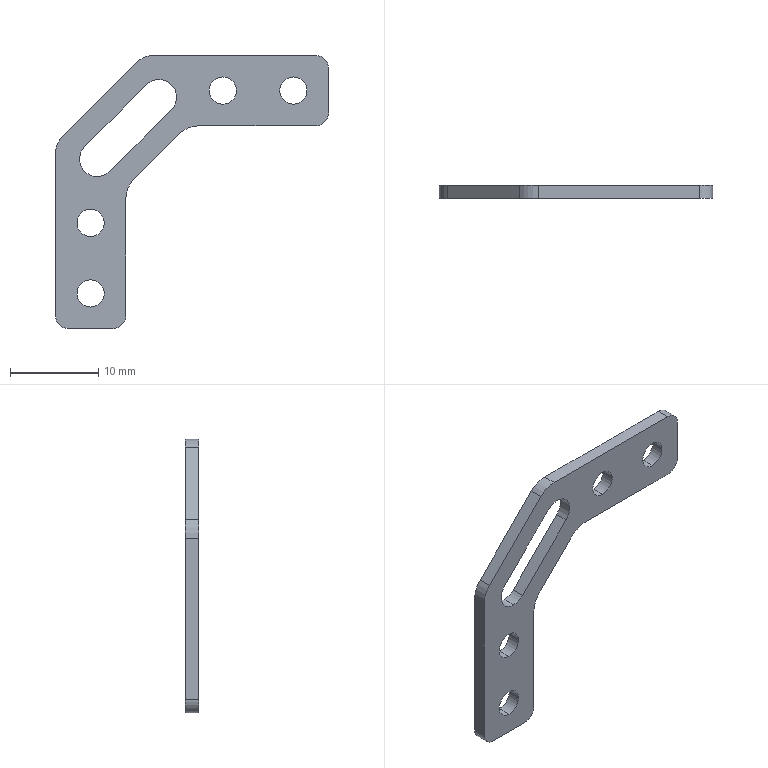Part | SolidWorks | features Fillet 2, Extrusion 1 | 1 solid | 31 faces | box 31 x 1.5 x 31 mm | volume 483.32 mm3 | cylinder 19 | plane 12 | commonest cylinder face diameters 3.1 x8 3 x4 6 x4 4 x3
STEP:
#1=CARTESIAN_POINT('',(2.164,1.5,-9.164));
#2=VERTEX_POINT('',#1);
#3=CARTESIAN_POINT('',(0.75,1.5,-9.75));
#4=VERTEX_POINT('',#3);
#5=CARTESIAN_POINT('',(0.75,1.5,-7.75));
#6=DIRECTION('',(0.,1.,0.));
#7=DIRECTION('',(0.,0.,1.));
#8=AXIS2_PLACEMENT_3D('',#5,#6,#7);
#9=CIRCLE('',#8,2.);
#10=EDGE_CURVE('',#2,#4,#9,.T.);
#11=ORIENTED_EDGE('',*,*,#10,.T.);
#12=CARTESIAN_POINT('',(0.75,0.,-9.75));
#13=VERTEX_POINT('',#12);
#14=CARTESIAN_POINT('',(0.75,1.5,-9.75));
#15=DIRECTION('',(0.,-1.,0.));
#16=VECTOR('',#15,1000.);
#17=LINE('',#14,#16);
#18=EDGE_CURVE('',#4,#13,#17,.T.);
#19=ORIENTED_EDGE('',*,*,#18,.T.);
#20=CARTESIAN_POINT('',(2.164,0.,-9.164));
#21=VERTEX_POINT('',#20);
#22=CARTESIAN_POINT('',(0.75,0.,-7.75));
#23=DIRECTION('',(0.,1.,0.));
#24=DIRECTION('',(0.,0.,1.));
#25=AXIS2_PLACEMENT_3D('',#22,#23,#24);
#26=CIRCLE('',#25,2.);
#27=EDGE_CURVE('',#21,#13,#26,.T.);
#28=ORIENTED_EDGE('',*,*,#27,.F.);
#29=CARTESIAN_POINT('',(2.164,1.5,-9.164));
#30=DIRECTION('',(0.,-1.,0.));
#31=VECTOR('',#30,1000.);
#32=LINE('',#29,#31);
#33=EDGE_CURVE('',#2,#21,#32,.T.);
#34=ORIENTED_EDGE('',*,*,#33,.F.);
#35=EDGE_LOOP('',(#11,#19,#28,#34));
#36=FACE_OUTER_BOUND('',#35,.T.);
#37=CARTESIAN_POINT('',(0.75,1.5,-7.75));
#38=DIRECTION('',(0.,-1.,0.));
#39=DIRECTION('',(0.,0.,-1.));
#40=AXIS2_PLACEMENT_3D('',#37,#38,#39);
#41=CYLINDRICAL_SURFACE('',#40,2.);
#42=ADVANCED_FACE('',(#36),#41,.F.);
#43=CARTESIAN_POINT('',(0.,1.5,-16.55));
#44=VERTEX_POINT('',#43);
#45=CARTESIAN_POINT('',(0.,1.5,-13.45));
#46=VERTEX_POINT('',#45);
#47=CARTESIAN_POINT('',(0.,1.5,-15.));
#48=DIRECTION('',(0.,1.,0.));
#49=DIRECTION('',(0.,0.,-1.));
#50=AXIS2_PLACEMENT_3D('',#47,#48,#49);
#51=CIRCLE('',#50,1.55);
#52=EDGE_CURVE('',#44,#46,#51,.T.);
#53=ORIENTED_EDGE('',*,*,#52,.T.);
#54=CARTESIAN_POINT('',(0.,0.,-13.45));
#55=VERTEX_POINT('',#54);
#56=CARTESIAN_POINT('',(0.,1.5,-13.45));
#57=DIRECTION('',(0.,-1.,0.));
#58=VECTOR('',#57,1000.);
#59=LINE('',#56,#58);
#60=EDGE_CURVE('',#46,#55,#59,.T.);
#61=ORIENTED_EDGE('',*,*,#60,.T.);
#62=CARTESIAN_POINT('',(0.,0.,-16.55));
#63=VERTEX_POINT('',#62);
#64=CARTESIAN_POINT('',(0.,0.,-15.));
#65=DIRECTION('',(0.,1.,0.));
#66=DIRECTION('',(0.,0.,-1.));
#67=AXIS2_PLACEMENT_3D('',#64,#65,#66);
#68=CIRCLE('',#67,1.55);
#69=EDGE_CURVE('',#63,#55,#68,.T.);
#70=ORIENTED_EDGE('',*,*,#69,.F.);
#71=CARTESIAN_POINT('',(0.,1.5,-16.55));
#72=DIRECTION('',(0.,-1.,0.));
#73=VECTOR('',#72,1000.);
#74=LINE('',#71,#73);
#75=EDGE_CURVE('',#44,#63,#74,.T.);
#76=ORIENTED_EDGE('',*,*,#75,.F.);
#77=EDGE_LOOP('',(#53,#61,#70,#76));
#78=FACE_OUTER_BOUND('',#77,.T.);
#79=CARTESIAN_POINT('',(0.,1.5,-15.));
#80=DIRECTION('',(0.,-1.,0.));
#81=DIRECTION('',(0.,0.,-1.));
#82=AXIS2_PLACEMENT_3D('',#79,#80,#81);
#83=CYLINDRICAL_SURFACE('',#82,1.55);
#84=ADVANCED_FACE('',(#78),#83,.F.);
#85=CARTESIAN_POINT('',(0.,1.5,-24.55));
#86=VERTEX_POINT('',#85);
#87=CARTESIAN_POINT('',(0.,1.5,-21.45));
#88=VERTEX_POINT('',#87);
#89=CARTESIAN_POINT('',(0.,1.5,-23.));
#90=DIRECTION('',(0.,1.,0.));
#91=DIRECTION('',(0.,0.,-1.));
#92=AXIS2_PLACEMENT_3D('',#89,#90,#91);
#93=CIRCLE('',#92,1.55);
#94=EDGE_CURVE('',#86,#88,#93,.T.);
#95=ORIENTED_EDGE('',*,*,#94,.T.);
#96=CARTESIAN_POINT('',(0.,0.,-21.45));
#97=VERTEX_POINT('',#96);
#98=CARTESIAN_POINT('',(0.,1.5,-21.45));
#99=DIRECTION('',(0.,-1.,0.));
#100=VECTOR('',#99,1000.);
#101=LINE('',#98,#100);
#102=EDGE_CURVE('',#88,#97,#101,.T.);
#103=ORIENTED_EDGE('',*,*,#102,.T.);
#104=CARTESIAN_POINT('',(0.,0.,-24.55));
#105=VERTEX_POINT('',#104);
#106=CARTESIAN_POINT('',(0.,0.,-23.));
#107=DIRECTION('',(0.,1.,0.));
#108=DIRECTION('',(0.,0.,-1.));
#109=AXIS2_PLACEMENT_3D('',#106,#107,#108);
#110=CIRCLE('',#109,1.55);
#111=EDGE_CURVE('',#105,#97,#110,.T.);
#112=ORIENTED_EDGE('',*,*,#111,.F.);
#113=CARTESIAN_POINT('',(0.,1.5,-24.55));
#114=DIRECTION('',(0.,-1.,0.));
#115=VECTOR('',#114,1000.);
#116=LINE('',#113,#115);
#117=EDGE_CURVE('',#86,#105,#116,.T.);
#118=ORIENTED_EDGE('',*,*,#117,.F.);
#119=EDGE_LOOP('',(#95,#103,#112,#118));
#120=FACE_OUTER_BOUND('',#119,.T.);
#121=CARTESIAN_POINT('',(0.,1.5,-23.));
#122=DIRECTION('',(0.,-1.,0.));
#123=DIRECTION('',(0.,0.,-1.));
#124=AXIS2_PLACEMENT_3D('',#121,#122,#123);
#125=CYLINDRICAL_SURFACE('',#124,1.55);
#126=ADVANCED_FACE('',(#120),#125,.F.);
#127=CARTESIAN_POINT('',(23.,1.5,-1.55));
#128=VERTEX_POINT('',#127);
#129=CARTESIAN_POINT('',(23.,1.5,1.55));
#130=VERTEX_POINT('',#129);
#131=CARTESIAN_POINT('',(23.,1.5,0.));
#132=DIRECTION('',(0.,1.,0.));
#133=DIRECTION('',(0.,0.,1.));
#134=AXIS2_PLACEMENT_3D('',#131,#132,#133);
#135=CIRCLE('',#134,1.55);
#136=EDGE_CURVE('',#128,#130,#135,.T.);
#137=ORIENTED_EDGE('',*,*,#136,.T.);
#138=CARTESIAN_POINT('',(23.,0.,1.55));
#139=VERTEX_POINT('',#138);
#140=CARTESIAN_POINT('',(23.,1.5,1.55));
#141=DIRECTION('',(0.,-1.,0.));
#142=VECTOR('',#141,1000.);
#143=LINE('',#140,#142);
#144=EDGE_CURVE('',#130,#139,#143,.T.);
#145=ORIENTED_EDGE('',*,*,#144,.T.);
#146=CARTESIAN_POINT('',(23.,0.,-1.55));
#147=VERTEX_POINT('',#146);
#148=CARTESIAN_POINT('',(23.,0.,0.));
#149=DIRECTION('',(0.,1.,0.));
#150=DIRECTION('',(0.,0.,1.));
#151=AXIS2_PLACEMENT_3D('',#148,#149,#150);
#152=CIRCLE('',#151,1.55);
#153=EDGE_CURVE('',#147,#139,#152,.T.);
#154=ORIENTED_EDGE('',*,*,#153,.F.);
#155=CARTESIAN_POINT('',(23.,1.5,-1.55));
#156=DIRECTION('',(0.,-1.,0.));
#157=VECTOR('',#156,1000.);
#158=LINE('',#155,#157);
#159=EDGE_CURVE('',#128,#147,#158,.T.);
#160=ORIENTED_EDGE('',*,*,#159,.F.);
#161=EDGE_LOOP('',(#137,#145,#154,#160));
#162=FACE_OUTER_BOUND('',#161,.T.);
#163=CARTESIAN_POINT('',(23.,1.5,0.));
#164=DIRECTION('',(0.,-1.,0.));
#165=DIRECTION('',(0.,0.,-1.));
#166=AXIS2_PLACEMENT_3D('',#163,#164,#165);
#167=CYLINDRICAL_SURFACE('',#166,1.55);
#168=ADVANCED_FACE('',(#162),#167,.F.);
#169=CARTESIAN_POINT('',(15.,1.5,-1.55));
#170=VERTEX_POINT('',#169);
#171=CARTESIAN_POINT('',(15.,1.5,1.55));
#172=VERTEX_POINT('',#171);
#173=CARTESIAN_POINT('',(15.,1.5,0.));
#174=DIRECTION('',(0.,1.,0.));
#175=DIRECTION('',(0.,0.,1.));
#176=AXIS2_PLACEMENT_3D('',#173,#174,#175);
#177=CIRCLE('',#176,1.55);
#178=EDGE_CURVE('',#170,#172,#177,.T.);
#179=ORIENTED_EDGE('',*,*,#178,.T.);
#180=CARTESIAN_POINT('',(15.,0.,1.55));
#181=VERTEX_POINT('',#180);
#182=CARTESIAN_POINT('',(15.,1.5,1.55));
#183=DIRECTION('',(0.,-1.,0.));
#184=VECTOR('',#183,1000.);
#185=LINE('',#182,#184);
#186=EDGE_CURVE('',#172,#181,#185,.T.);
#187=ORIENTED_EDGE('',*,*,#186,.T.);
#188=CARTESIAN_POINT('',(15.,0.,-1.55));
#189=VERTEX_POINT('',#188);
#190=CARTESIAN_POINT('',(15.,0.,0.));
#191=DIRECTION('',(0.,1.,0.));
#192=DIRECTION('',(0.,0.,1.));
#193=AXIS2_PLACEMENT_3D('',#190,#191,#192);
#194=CIRCLE('',#193,1.55);
#195=EDGE_CURVE('',#189,#181,#194,.T.);
#196=ORIENTED_EDGE('',*,*,#195,.F.);
#197=CARTESIAN_POINT('',(15.,1.5,-1.55));
#198=DIRECTION('',(0.,-1.,0.));
#199=VECTOR('',#198,1000.);
#200=LINE('',#197,#199);
#201=EDGE_CURVE('',#170,#189,#200,.T.);
#202=ORIENTED_EDGE('',*,*,#201,.F.);
#203=EDGE_LOOP('',(#179,#187,#196,#202));
#204=FACE_OUTER_BOUND('',#203,.T.);
#205=CARTESIAN_POINT('',(15.,1.5,0.));
#206=DIRECTION('',(0.,-1.,0.));
#207=DIRECTION('',(0.,0.,-1.));
#208=AXIS2_PLACEMENT_3D('',#205,#206,#207);
#209=CYLINDRICAL_SURFACE('',#208,1.55);
#210=ADVANCED_FACE('',(#204),#209,.F.);
#211=ORIENTED_EDGE('',*,*,#94,.F.);
#212=CARTESIAN_POINT('',(0.,1.5,-23.));
#213=DIRECTION('',(0.,1.,0.));
#214=DIRECTION('',(0.,0.,-1.));
#215=AXIS2_PLACEMENT_3D('',#212,#213,#214);
#216=CIRCLE('',#215,1.55);
#217=EDGE_CURVE('',#88,#86,#216,.T.);
#218=ORIENTED_EDGE('',*,*,#217,.F.);
#219=EDGE_LOOP('',(#211,#218));
#220=FACE_BOUND('',#219,.T.);
#221=ORIENTED_EDGE('',*,*,#178,.F.);
#222=CARTESIAN_POINT('',(15.,1.5,0.));
#223=DIRECTION('',(0.,1.,0.));
#224=DIRECTION('',(0.,0.,1.));
#225=AXIS2_PLACEMENT_3D('',#222,#223,#224);
#226=CIRCLE('',#225,1.55);
#227=EDGE_CURVE('',#172,#170,#226,.T.);
#228=ORIENTED_EDGE('',*,*,#227,.F.);
#229=EDGE_LOOP('',(#221,#228));
#230=FACE_BOUND('',#229,.T.);
#231=CARTESIAN_POINT('',(-3.121,1.5,-5.121));
#232=VERTEX_POINT('',#231);
#233=CARTESIAN_POINT('',(5.121,1.5,3.121));
#234=VERTEX_POINT('',#233);
#235=CARTESIAN_POINT('',(6.,1.5,4.));
#236=DIRECTION('',(0.7071,0.,0.7071));
#237=VECTOR('',#236,1000.);
#238=LINE('',#235,#237);
#239=EDGE_CURVE('',#232,#234,#238,.T.);
#240=ORIENTED_EDGE('',*,*,#239,.T.);
#241=CARTESIAN_POINT('',(7.243,1.5,4.));
#242=VERTEX_POINT('',#241);
#243=CARTESIAN_POINT('',(7.243,1.5,1.));
#244=DIRECTION('',(0.,1.,0.));
#245=DIRECTION('',(0.,0.,1.));
#246=AXIS2_PLACEMENT_3D('',#243,#244,#245);
#247=CIRCLE('',#246,3.);
#248=EDGE_CURVE('',#234,#242,#247,.T.);
#249=ORIENTED_EDGE('',*,*,#248,.T.);
#250=CARTESIAN_POINT('',(25.5,1.5,4.));
#251=VERTEX_POINT('',#250);
#252=CARTESIAN_POINT('',(27.,1.5,4.));
#253=DIRECTION('',(1.,0.,0.));
#254=VECTOR('',#253,1000.);
#255=LINE('',#252,#254);
#256=EDGE_CURVE('',#242,#251,#255,.T.);
#257=ORIENTED_EDGE('',*,*,#256,.T.);
#258=CARTESIAN_POINT('',(27.,1.5,2.5));
#259=VERTEX_POINT('',#258);
#260=CARTESIAN_POINT('',(25.5,1.5,2.5));
#261=DIRECTION('',(0.,1.,0.));
#262=DIRECTION('',(0.,0.,1.));
#263=AXIS2_PLACEMENT_3D('',#260,#261,#262);
#264=CIRCLE('',#263,1.5);
#265=EDGE_CURVE('',#251,#259,#264,.T.);
#266=ORIENTED_EDGE('',*,*,#265,.T.);
#267=CARTESIAN_POINT('',(27.,1.5,-2.5));
#268=VERTEX_POINT('',#267);
#269=CARTESIAN_POINT('',(27.,1.5,4.));
#270=DIRECTION('',(0.,0.,-1.));
#271=VECTOR('',#270,1000.);
#272=LINE('',#269,#271);
#273=EDGE_CURVE('',#259,#268,#272,.T.);
#274=ORIENTED_EDGE('',*,*,#273,.T.);
#275=CARTESIAN_POINT('',(25.5,1.5,-4.));
#276=VERTEX_POINT('',#275);
#277=CARTESIAN_POINT('',(25.5,1.5,-2.5));
#278=DIRECTION('',(0.,1.,0.));
#279=DIRECTION('',(0.,0.,1.));
#280=AXIS2_PLACEMENT_3D('',#277,#278,#279);
#281=CIRCLE('',#280,1.5);
#282=EDGE_CURVE('',#268,#276,#281,.T.);
#283=ORIENTED_EDGE('',*,*,#282,.T.);
#284=CARTESIAN_POINT('',(12.243,1.5,-4.));
#285=VERTEX_POINT('',#284);
#286=CARTESIAN_POINT('',(27.,1.5,-4.));
#287=DIRECTION('',(-1.,0.,0.));
#288=VECTOR('',#287,1000.);
#289=LINE('',#286,#288);
#290=EDGE_CURVE('',#276,#285,#289,.T.);
#291=ORIENTED_EDGE('',*,*,#290,.T.);
#292=CARTESIAN_POINT('',(10.121,1.5,-4.879));
#293=VERTEX_POINT('',#292);
#294=CARTESIAN_POINT('',(12.243,1.5,-7.));
#295=DIRECTION('',(0.,-1.,0.));
#296=DIRECTION('',(0.,0.,1.));
#297=AXIS2_PLACEMENT_3D('',#294,#295,#296);
#298=CIRCLE('',#297,3.);
#299=EDGE_CURVE('',#285,#293,#298,.T.);
#300=ORIENTED_EDGE('',*,*,#299,.T.);
#301=CARTESIAN_POINT('',(4.879,1.5,-10.121));
#302=VERTEX_POINT('',#301);
#303=CARTESIAN_POINT('',(11.,1.5,-4.));
#304=DIRECTION('',(-0.7071,0.,-0.7071));
#305=VECTOR('',#304,1000.);
#306=LINE('',#303,#305);
#307=EDGE_CURVE('',#293,#302,#306,.T.);
#308=ORIENTED_EDGE('',*,*,#307,.T.);
#309=CARTESIAN_POINT('',(4.,1.5,-12.243));
#310=VERTEX_POINT('',#309);
#311=CARTESIAN_POINT('',(7.,1.5,-12.243));
#312=DIRECTION('',(0.,-1.,0.));
#313=DIRECTION('',(0.,0.,1.));
#314=AXIS2_PLACEMENT_3D('',#311,#312,#313);
#315=CIRCLE('',#314,3.);
#316=EDGE_CURVE('',#302,#310,#315,.T.);
#317=ORIENTED_EDGE('',*,*,#316,.T.);
#318=CARTESIAN_POINT('',(4.,1.5,-25.5));
#319=VERTEX_POINT('',#318);
#320=CARTESIAN_POINT('',(4.,1.5,-27.));
#321=DIRECTION('',(0.,0.,-1.));
#322=VECTOR('',#321,1000.);
#323=LINE('',#320,#322);
#324=EDGE_CURVE('',#310,#319,#323,.T.);
#325=ORIENTED_EDGE('',*,*,#324,.T.);
#326=CARTESIAN_POINT('',(2.5,1.5,-27.));
#327=VERTEX_POINT('',#326);
#328=CARTESIAN_POINT('',(2.5,1.5,-25.5));
#329=DIRECTION('',(0.,1.,0.));
#330=DIRECTION('',(0.,0.,1.));
#331=AXIS2_PLACEMENT_3D('',#328,#329,#330);
#332=CIRCLE('',#331,1.5);
#333=EDGE_CURVE('',#319,#327,#332,.T.);
#334=ORIENTED_EDGE('',*,*,#333,.T.);
#335=CARTESIAN_POINT('',(-2.5,1.5,-27.));
#336=VERTEX_POINT('',#335);
#337=CARTESIAN_POINT('',(-4.,1.5,-27.));
#338=DIRECTION('',(-1.,0.,0.));
#339=VECTOR('',#338,1000.);
#340=LINE('',#337,#339);
#341=EDGE_CURVE('',#327,#336,#340,.T.);
#342=ORIENTED_EDGE('',*,*,#341,.T.);
#343=CARTESIAN_POINT('',(-4.,1.5,-25.5));
#344=VERTEX_POINT('',#343);
#345=CARTESIAN_POINT('',(-2.5,1.5,-25.5));
#346=DIRECTION('',(0.,1.,0.));
#347=DIRECTION('',(0.,0.,1.));
#348=AXIS2_PLACEMENT_3D('',#345,#346,#347);
#349=CIRCLE('',#348,1.5);
#350=EDGE_CURVE('',#336,#344,#349,.T.);
#351=ORIENTED_EDGE('',*,*,#350,.T.);
#352=CARTESIAN_POINT('',(-4.,1.5,-7.243));
#353=VERTEX_POINT('',#352);
#354=CARTESIAN_POINT('',(-4.,1.5,-27.));
#355=DIRECTION('',(0.,0.,1.));
#356=VECTOR('',#355,1000.);
#357=LINE('',#354,#356);
#358=EDGE_CURVE('',#344,#353,#357,.T.);
#359=ORIENTED_EDGE('',*,*,#358,.T.);
#360=CARTESIAN_POINT('',(-1.,1.5,-7.243));
#361=DIRECTION('',(0.,1.,0.));
#362=DIRECTION('',(0.,0.,1.));
#363=AXIS2_PLACEMENT_3D('',#360,#361,#362);
#364=CIRCLE('',#363,3.);
#365=EDGE_CURVE('',#353,#232,#364,.T.);
#366=ORIENTED_EDGE('',*,*,#365,.T.);
#367=EDGE_LOOP('',(#240,#249,#257,#266,#274,#283,#291,#300,#308,#317,#325,#334,#342,#351,#359,#366));
#368=FACE_OUTER_BOUND('',#367,.T.);
#369=ORIENTED_EDGE('',*,*,#136,.F.);
#370=CARTESIAN_POINT('',(23.,1.5,0.));
#371=DIRECTION('',(0.,1.,0.));
#372=DIRECTION('',(0.,0.,1.));
#373=AXIS2_PLACEMENT_3D('',#370,#371,#372);
#374=CIRCLE('',#373,1.55);
#375=EDGE_CURVE('',#130,#128,#374,.T.);
#376=ORIENTED_EDGE('',*,*,#375,.F.);
#377=EDGE_LOOP('',(#369,#376));
#378=FACE_BOUND('',#377,.T.);
#379=ORIENTED_EDGE('',*,*,#52,.F.);
#380=CARTESIAN_POINT('',(0.,1.5,-15.));
#381=DIRECTION('',(0.,1.,0.));
#382=DIRECTION('',(0.,0.,-1.));
#383=AXIS2_PLACEMENT_3D('',#380,#381,#382);
#384=CIRCLE('',#383,1.55);
#385=EDGE_CURVE('',#46,#44,#384,.T.);
#386=ORIENTED_EDGE('',*,*,#385,.F.);
#387=EDGE_LOOP('',(#379,#386));
#388=FACE_BOUND('',#387,.T.);
#389=CARTESIAN_POINT('',(-0.6642,1.5,-6.336));
#390=VERTEX_POINT('',#389);
#391=CARTESIAN_POINT('',(6.336,1.5,0.6642));
#392=VERTEX_POINT('',#391);
#393=CARTESIAN_POINT('',(-0.6642,1.5,-6.336));
#394=DIRECTION('',(0.7071,0.,0.7071));
#395=VECTOR('',#394,1000.);
#396=LINE('',#393,#395);
#397=EDGE_CURVE('',#390,#392,#396,.T.);
#398=ORIENTED_EDGE('',*,*,#397,.F.);
#399=CARTESIAN_POINT('',(0.75,1.5,-7.75));
#400=DIRECTION('',(0.,1.,0.));
#401=DIRECTION('',(0.,0.,1.));
#402=AXIS2_PLACEMENT_3D('',#399,#400,#401);
#403=CIRCLE('',#402,2.);
#404=EDGE_CURVE('',#4,#390,#403,.T.);
#405=ORIENTED_EDGE('',*,*,#404,.F.);
#406=ORIENTED_EDGE('',*,*,#10,.F.);
#407=CARTESIAN_POINT('',(9.164,1.5,-2.164));
#408=VERTEX_POINT('',#407);
#409=CARTESIAN_POINT('',(2.164,1.5,-9.164));
#410=DIRECTION('',(-0.7071,0.,-0.7071));
#411=VECTOR('',#410,1000.);
#412=LINE('',#409,#411);
#413=EDGE_CURVE('',#408,#2,#412,.T.);
#414=ORIENTED_EDGE('',*,*,#413,.F.);
#415=CARTESIAN_POINT('',(7.75,1.5,-0.75));
#416=DIRECTION('',(0.,1.,0.));
#417=DIRECTION('',(0.,0.,1.));
#418=AXIS2_PLACEMENT_3D('',#415,#416,#417);
#419=CIRCLE('',#418,2.);
#420=EDGE_CURVE('',#392,#408,#419,.T.);
#421=ORIENTED_EDGE('',*,*,#420,.F.);
#422=EDGE_LOOP('',(#398,#405,#406,#414,#421));
#423=FACE_BOUND('',#422,.T.);
#424=CARTESIAN_POINT('',(0.,1.5,0.));
#425=DIRECTION('',(0.,1.,0.));
#426=DIRECTION('',(0.,0.,1.));
#427=AXIS2_PLACEMENT_3D('',#424,#425,#426);
#428=PLANE('',#427);
#429=ADVANCED_FACE('',(#220,#230,#368,#378,#388,#423),#428,.T.);
#430=ORIENTED_EDGE('',*,*,#69,.T.);
#431=CARTESIAN_POINT('',(0.,0.,-15.));
#432=DIRECTION('',(0.,1.,0.));
#433=DIRECTION('',(0.,0.,-1.));
#434=AXIS2_PLACEMENT_3D('',#431,#432,#433);
#435=CIRCLE('',#434,1.55);
#436=EDGE_CURVE('',#55,#63,#435,.T.);
#437=ORIENTED_EDGE('',*,*,#436,.T.);
#438=EDGE_LOOP('',(#430,#437));
#439=FACE_BOUND('',#438,.T.);
#440=ORIENTED_EDGE('',*,*,#111,.T.);
#441=CARTESIAN_POINT('',(0.,0.,-23.));
#442=DIRECTION('',(0.,1.,0.));
#443=DIRECTION('',(0.,0.,-1.));
#444=AXIS2_PLACEMENT_3D('',#441,#442,#443);
#445=CIRCLE('',#444,1.55);
#446=EDGE_CURVE('',#97,#105,#445,.T.);
#447=ORIENTED_EDGE('',*,*,#446,.T.);
#448=EDGE_LOOP('',(#440,#447));
#449=FACE_BOUND('',#448,.T.);
#450=ORIENTED_EDGE('',*,*,#153,.T.);
#451=CARTESIAN_POINT('',(23.,0.,0.));
#452=DIRECTION('',(0.,1.,0.));
#453=DIRECTION('',(0.,0.,1.));
#454=AXIS2_PLACEMENT_3D('',#451,#452,#453);
#455=CIRCLE('',#454,1.55);
#456=EDGE_CURVE('',#139,#147,#455,.T.);
#457=ORIENTED_EDGE('',*,*,#456,.T.);
#458=EDGE_LOOP('',(#450,#457));
#459=FACE_BOUND('',#458,.T.);
#460=ORIENTED_EDGE('',*,*,#195,.T.);
#461=CARTESIAN_POINT('',(15.,0.,0.));
#462=DIRECTION('',(0.,1.,0.));
#463=DIRECTION('',(0.,0.,1.));
#464=AXIS2_PLACEMENT_3D('',#461,#462,#463);
#465=CIRCLE('',#464,1.55);
#466=EDGE_CURVE('',#181,#189,#465,.T.);
#467=ORIENTED_EDGE('',*,*,#466,.T.);
#468=EDGE_LOOP('',(#460,#467));
#469=FACE_BOUND('',#468,.T.);
#470=CARTESIAN_POINT('',(7.243,0.,4.));
#471=VERTEX_POINT('',#470);
#472=CARTESIAN_POINT('',(25.5,0.,4.));
#473=VERTEX_POINT('',#472);
#474=CARTESIAN_POINT('',(27.,0.,4.));
#475=DIRECTION('',(1.,0.,0.));
#476=VECTOR('',#475,1000.);
#477=LINE('',#474,#476);
#478=EDGE_CURVE('',#471,#473,#477,.T.);
#479=ORIENTED_EDGE('',*,*,#478,.F.);
#480=CARTESIAN_POINT('',(5.121,0.,3.121));
#481=VERTEX_POINT('',#480);
#482=CARTESIAN_POINT('',(7.243,0.,1.));
#483=DIRECTION('',(0.,-1.,0.));
#484=DIRECTION('',(0.,0.,1.));
#485=AXIS2_PLACEMENT_3D('',#482,#483,#484);
#486=CIRCLE('',#485,3.);
#487=EDGE_CURVE('',#471,#481,#486,.T.);
#488=ORIENTED_EDGE('',*,*,#487,.T.);
#489=CARTESIAN_POINT('',(-3.121,0.,-5.121));
#490=VERTEX_POINT('',#489);
#491=CARTESIAN_POINT('',(6.,0.,4.));
#492=DIRECTION('',(0.7071,0.,0.7071));
#493=VECTOR('',#492,1000.);
#494=LINE('',#491,#493);
#495=EDGE_CURVE('',#490,#481,#494,.T.);
#496=ORIENTED_EDGE('',*,*,#495,.F.);
#497=CARTESIAN_POINT('',(-4.,0.,-7.243));
#498=VERTEX_POINT('',#497);
#499=CARTESIAN_POINT('',(-1.,0.,-7.243));
#500=DIRECTION('',(0.,-1.,0.));
#501=DIRECTION('',(0.,0.,1.));
#502=AXIS2_PLACEMENT_3D('',#499,#500,#501);
#503=CIRCLE('',#502,3.);
#504=EDGE_CURVE('',#490,#498,#503,.T.);
#505=ORIENTED_EDGE('',*,*,#504,.T.);
#506=CARTESIAN_POINT('',(-4.,0.,-25.5));
#507=VERTEX_POINT('',#506);
#508=CARTESIAN_POINT('',(-4.,0.,-27.));
#509=DIRECTION('',(0.,0.,1.));
#510=VECTOR('',#509,1000.);
#511=LINE('',#508,#510);
#512=EDGE_CURVE('',#507,#498,#511,.T.);
#513=ORIENTED_EDGE('',*,*,#512,.F.);
#514=CARTESIAN_POINT('',(-2.5,0.,-27.));
#515=VERTEX_POINT('',#514);
#516=CARTESIAN_POINT('',(-2.5,0.,-25.5));
#517=DIRECTION('',(0.,-1.,0.));
#518=DIRECTION('',(0.,0.,1.));
#519=AXIS2_PLACEMENT_3D('',#516,#517,#518);
#520=CIRCLE('',#519,1.5);
#521=EDGE_CURVE('',#507,#515,#520,.T.);
#522=ORIENTED_EDGE('',*,*,#521,.T.);
#523=CARTESIAN_POINT('',(2.5,0.,-27.));
#524=VERTEX_POINT('',#523);
#525=CARTESIAN_POINT('',(-4.,0.,-27.));
#526=DIRECTION('',(-1.,0.,0.));
#527=VECTOR('',#526,1000.);
#528=LINE('',#525,#527);
#529=EDGE_CURVE('',#524,#515,#528,.T.);
#530=ORIENTED_EDGE('',*,*,#529,.F.);
#531=CARTESIAN_POINT('',(4.,0.,-25.5));
#532=VERTEX_POINT('',#531);
#533=CARTESIAN_POINT('',(2.5,0.,-25.5));
#534=DIRECTION('',(0.,-1.,0.));
#535=DIRECTION('',(0.,0.,1.));
#536=AXIS2_PLACEMENT_3D('',#533,#534,#535);
#537=CIRCLE('',#536,1.5);
#538=EDGE_CURVE('',#524,#532,#537,.T.);
#539=ORIENTED_EDGE('',*,*,#538,.T.);
#540=CARTESIAN_POINT('',(4.,0.,-12.243));
#541=VERTEX_POINT('',#540);
#542=CARTESIAN_POINT('',(4.,0.,-27.));
#543=DIRECTION('',(0.,0.,-1.));
#544=VECTOR('',#543,1000.);
#545=LINE('',#542,#544);
#546=EDGE_CURVE('',#541,#532,#545,.T.);
#547=ORIENTED_EDGE('',*,*,#546,.F.);
#548=CARTESIAN_POINT('',(4.879,0.,-10.121));
#549=VERTEX_POINT('',#548);
#550=CARTESIAN_POINT('',(7.,0.,-12.243));
#551=DIRECTION('',(0.,1.,0.));
#552=DIRECTION('',(0.,0.,1.));
#553=AXIS2_PLACEMENT_3D('',#550,#551,#552);
#554=CIRCLE('',#553,3.);
#555=EDGE_CURVE('',#541,#549,#554,.T.);
#556=ORIENTED_EDGE('',*,*,#555,.T.);
#557=CARTESIAN_POINT('',(10.121,0.,-4.879));
#558=VERTEX_POINT('',#557);
#559=CARTESIAN_POINT('',(11.,0.,-4.));
#560=DIRECTION('',(-0.7071,0.,-0.7071));
#561=VECTOR('',#560,1000.);
#562=LINE('',#559,#561);
#563=EDGE_CURVE('',#558,#549,#562,.T.);
#564=ORIENTED_EDGE('',*,*,#563,.F.);
#565=CARTESIAN_POINT('',(12.243,0.,-4.));
#566=VERTEX_POINT('',#565);
#567=CARTESIAN_POINT('',(12.243,0.,-7.));
#568=DIRECTION('',(0.,1.,0.));
#569=DIRECTION('',(0.,0.,1.));
#570=AXIS2_PLACEMENT_3D('',#567,#568,#569);
#571=CIRCLE('',#570,3.);
#572=EDGE_CURVE('',#558,#566,#571,.T.);
#573=ORIENTED_EDGE('',*,*,#572,.T.);
#574=CARTESIAN_POINT('',(25.5,0.,-4.));
#575=VERTEX_POINT('',#574);
#576=CARTESIAN_POINT('',(27.,0.,-4.));
#577=DIRECTION('',(-1.,0.,0.));
#578=VECTOR('',#577,1000.);
#579=LINE('',#576,#578);
#580=EDGE_CURVE('',#575,#566,#579,.T.);
#581=ORIENTED_EDGE('',*,*,#580,.F.);
#582=CARTESIAN_POINT('',(27.,0.,-2.5));
#583=VERTEX_POINT('',#582);
#584=CARTESIAN_POINT('',(25.5,0.,-2.5));
#585=DIRECTION('',(0.,-1.,0.));
#586=DIRECTION('',(0.,0.,1.));
#587=AXIS2_PLACEMENT_3D('',#584,#585,#586);
#588=CIRCLE('',#587,1.5);
#589=EDGE_CURVE('',#575,#583,#588,.T.);
#590=ORIENTED_EDGE('',*,*,#589,.T.);
#591=CARTESIAN_POINT('',(27.,0.,2.5));
#592=VERTEX_POINT('',#591);
#593=CARTESIAN_POINT('',(27.,0.,4.));
#594=DIRECTION('',(0.,0.,-1.));
#595=VECTOR('',#594,1000.);
#596=LINE('',#593,#595);
#597=EDGE_CURVE('',#592,#583,#596,.T.);
#598=ORIENTED_EDGE('',*,*,#597,.F.);
#599=CARTESIAN_POINT('',(25.5,0.,2.5));
#600=DIRECTION('',(0.,-1.,0.));
#601=DIRECTION('',(0.,0.,1.));
#602=AXIS2_PLACEMENT_3D('',#599,#600,#601);
#603=CIRCLE('',#602,1.5);
#604=EDGE_CURVE('',#592,#473,#603,.T.);
#605=ORIENTED_EDGE('',*,*,#604,.T.);
#606=EDGE_LOOP('',(#479,#488,#496,#505,#513,#522,#530,#539,#547,#556,#564,#573,#581,#590,#598,#605));
#607=FACE_OUTER_BOUND('',#606,.T.);
#608=ORIENTED_EDGE('',*,*,#27,.T.);
#609=CARTESIAN_POINT('',(-0.6642,0.,-6.336));
#610=VERTEX_POINT('',#609);
#611=CARTESIAN_POINT('',(0.75,0.,-7.75));
#612=DIRECTION('',(0.,1.,0.));
#613=DIRECTION('',(0.,0.,1.));
#614=AXIS2_PLACEMENT_3D('',#611,#612,#613);
#615=CIRCLE('',#614,2.);
#616=EDGE_CURVE('',#13,#610,#615,.T.);
#617=ORIENTED_EDGE('',*,*,#616,.T.);
#618=CARTESIAN_POINT('',(6.336,0.,0.6642));
#619=VERTEX_POINT('',#618);
#620=CARTESIAN_POINT('',(-0.6642,0.,-6.336));
#621=DIRECTION('',(0.7071,0.,0.7071));
#622=VECTOR('',#621,1000.);
#623=LINE('',#620,#622);
#624=EDGE_CURVE('',#610,#619,#623,.T.);
#625=ORIENTED_EDGE('',*,*,#624,.T.);
#626=CARTESIAN_POINT('',(9.164,0.,-2.164));
#627=VERTEX_POINT('',#626);
#628=CARTESIAN_POINT('',(7.75,0.,-0.75));
#629=DIRECTION('',(0.,1.,0.));
#630=DIRECTION('',(0.,0.,1.));
#631=AXIS2_PLACEMENT_3D('',#628,#629,#630);
#632=CIRCLE('',#631,2.);
#633=EDGE_CURVE('',#619,#627,#632,.T.);
#634=ORIENTED_EDGE('',*,*,#633,.T.);
#635=CARTESIAN_POINT('',(2.164,0.,-9.164));
#636=DIRECTION('',(-0.7071,0.,-0.7071));
#637=VECTOR('',#636,1000.);
#638=LINE('',#635,#637);
#639=EDGE_CURVE('',#627,#21,#638,.T.);
#640=ORIENTED_EDGE('',*,*,#639,.T.);
#641=EDGE_LOOP('',(#608,#617,#625,#634,#640));
#642=FACE_BOUND('',#641,.T.);
#643=CARTESIAN_POINT('',(0.,0.,0.));
#644=DIRECTION('',(0.,1.,0.));
#645=DIRECTION('',(0.,0.,1.));
#646=AXIS2_PLACEMENT_3D('',#643,#644,#645);
#647=PLANE('',#646);
#648=ADVANCED_FACE('',(#439,#449,#459,#469,#607,#642),#647,.F.);
#649=ORIENTED_EDGE('',*,*,#256,.F.);
#650=CARTESIAN_POINT('',(7.243,1.5,4.));
#651=DIRECTION('',(0.,-1.,0.));
#652=VECTOR('',#651,1000.);
#653=LINE('',#650,#652);
#654=EDGE_CURVE('',#242,#471,#653,.T.);
#655=ORIENTED_EDGE('',*,*,#654,.T.);
#656=ORIENTED_EDGE('',*,*,#478,.T.);
#657=CARTESIAN_POINT('',(25.5,1.5,4.));
#658=DIRECTION('',(0.,1.,0.));
#659=VECTOR('',#658,1000.);
#660=LINE('',#657,#659);
#661=EDGE_CURVE('',#473,#251,#660,.T.);
#662=ORIENTED_EDGE('',*,*,#661,.T.);
#663=EDGE_LOOP('',(#649,#655,#656,#662));
#664=FACE_OUTER_BOUND('',#663,.T.);
#665=CARTESIAN_POINT('',(27.,1.5,4.));
#666=DIRECTION('',(0.,0.,-1.));
#667=DIRECTION('',(-1.,0.,0.));
#668=AXIS2_PLACEMENT_3D('',#665,#666,#667);
#669=PLANE('',#668);
#670=ADVANCED_FACE('',(#664),#669,.F.);
#671=ORIENTED_EDGE('',*,*,#273,.F.);
#672=CARTESIAN_POINT('',(27.,1.5,2.5));
#673=DIRECTION('',(0.,-1.,0.));
#674=VECTOR('',#673,1000.);
#675=LINE('',#672,#674);
#676=EDGE_CURVE('',#259,#592,#675,.T.);
#677=ORIENTED_EDGE('',*,*,#676,.T.);
#678=ORIENTED_EDGE('',*,*,#597,.T.);
#679=CARTESIAN_POINT('',(27.,1.5,-2.5));
#680=DIRECTION('',(0.,1.,0.));
#681=VECTOR('',#680,1000.);
#682=LINE('',#679,#681);
#683=EDGE_CURVE('',#583,#268,#682,.T.);
#684=ORIENTED_EDGE('',*,*,#683,.T.);
#685=EDGE_LOOP('',(#671,#677,#678,#684));
#686=FACE_OUTER_BOUND('',#685,.T.);
#687=CARTESIAN_POINT('',(27.,1.5,4.));
#688=DIRECTION('',(-1.,0.,0.));
#689=DIRECTION('',(0.,0.,1.));
#690=AXIS2_PLACEMENT_3D('',#687,#688,#689);
#691=PLANE('',#690);
#692=ADVANCED_FACE('',(#686),#691,.F.);
#693=ORIENTED_EDGE('',*,*,#580,.T.);
#694=CARTESIAN_POINT('',(12.243,1.5,-4.));
#695=DIRECTION('',(0.,1.,0.));
#696=VECTOR('',#695,1000.);
#697=LINE('',#694,#696);
#698=EDGE_CURVE('',#566,#285,#697,.T.);
#699=ORIENTED_EDGE('',*,*,#698,.T.);
#700=ORIENTED_EDGE('',*,*,#290,.F.);
#701=CARTESIAN_POINT('',(25.5,1.5,-4.));
#702=DIRECTION('',(0.,-1.,0.));
#703=VECTOR('',#702,1000.);
#704=LINE('',#701,#703);
#705=EDGE_CURVE('',#276,#575,#704,.T.);
#706=ORIENTED_EDGE('',*,*,#705,.T.);
#707=EDGE_LOOP('',(#693,#699,#700,#706));
#708=FACE_OUTER_BOUND('',#707,.T.);
#709=CARTESIAN_POINT('',(27.,1.5,-4.));
#710=DIRECTION('',(0.,0.,1.));
#711=DIRECTION('',(1.,0.,0.));
#712=AXIS2_PLACEMENT_3D('',#709,#710,#711);
#713=PLANE('',#712);
#714=ADVANCED_FACE('',(#708),#713,.F.);
#715=ORIENTED_EDGE('',*,*,#563,.T.);
#716=CARTESIAN_POINT('',(4.879,1.5,-10.121));
#717=DIRECTION('',(0.,1.,0.));
#718=VECTOR('',#717,1000.);
#719=LINE('',#716,#718);
#720=EDGE_CURVE('',#549,#302,#719,.T.);
#721=ORIENTED_EDGE('',*,*,#720,.T.);
#722=ORIENTED_EDGE('',*,*,#307,.F.);
#723=CARTESIAN_POINT('',(10.121,0.,-4.879));
#724=DIRECTION('',(0.,-1.,0.));
#725=VECTOR('',#724,1000.);
#726=LINE('',#723,#725);
#727=EDGE_CURVE('',#293,#558,#726,.T.);
#728=ORIENTED_EDGE('',*,*,#727,.T.);
#729=EDGE_LOOP('',(#715,#721,#722,#728));
#730=FACE_OUTER_BOUND('',#729,.T.);
#731=CARTESIAN_POINT('',(11.,1.5,-4.));
#732=DIRECTION('',(-0.7071,0.,0.7071));
#733=DIRECTION('',(0.7071,0.,0.7071));
#734=AXIS2_PLACEMENT_3D('',#731,#732,#733);
#735=PLANE('',#734);
#736=ADVANCED_FACE('',(#730),#735,.F.);
#737=ORIENTED_EDGE('',*,*,#324,.F.);
#738=CARTESIAN_POINT('',(4.,0.,-12.243));
#739=DIRECTION('',(0.,-1.,0.));
#740=VECTOR('',#739,1000.);
#741=LINE('',#738,#740);
#742=EDGE_CURVE('',#310,#541,#741,.T.);
#743=ORIENTED_EDGE('',*,*,#742,.T.);
#744=ORIENTED_EDGE('',*,*,#546,.T.);
#745=CARTESIAN_POINT('',(4.,1.5,-25.5));
#746=DIRECTION('',(0.,1.,0.));
#747=VECTOR('',#746,1000.);
#748=LINE('',#745,#747);
#749=EDGE_CURVE('',#532,#319,#748,.T.);
#750=ORIENTED_EDGE('',*,*,#749,.T.);
#751=EDGE_LOOP('',(#737,#743,#744,#750));
#752=FACE_OUTER_BOUND('',#751,.T.);
#753=CARTESIAN_POINT('',(4.,1.5,-27.));
#754=DIRECTION('',(-1.,0.,0.));
#755=DIRECTION('',(0.,0.,1.));
#756=AXIS2_PLACEMENT_3D('',#753,#754,#755);
#757=PLANE('',#756);
#758=ADVANCED_FACE('',(#752),#757,.F.);
#759=ORIENTED_EDGE('',*,*,#341,.F.);
#760=CARTESIAN_POINT('',(2.5,1.5,-27.));
#761=DIRECTION('',(0.,-1.,0.));
#762=VECTOR('',#761,1000.);
#763=LINE('',#760,#762);
#764=EDGE_CURVE('',#327,#524,#763,.T.);
#765=ORIENTED_EDGE('',*,*,#764,.T.);
#766=ORIENTED_EDGE('',*,*,#529,.T.);
#767=CARTESIAN_POINT('',(-2.5,1.5,-27.));
#768=DIRECTION('',(0.,1.,0.));
#769=VECTOR('',#768,1000.);
#770=LINE('',#767,#769);
#771=EDGE_CURVE('',#515,#336,#770,.T.);
#772=ORIENTED_EDGE('',*,*,#771,.T.);
#773=EDGE_LOOP('',(#759,#765,#766,#772));
#774=FACE_OUTER_BOUND('',#773,.T.);
#775=CARTESIAN_POINT('',(-4.,1.5,-27.));
#776=DIRECTION('',(0.,0.,1.));
#777=DIRECTION('',(1.,0.,0.));
#778=AXIS2_PLACEMENT_3D('',#775,#776,#777);
#779=PLANE('',#778);
#780=ADVANCED_FACE('',(#774),#779,.F.);
#781=ORIENTED_EDGE('',*,*,#512,.T.);
#782=CARTESIAN_POINT('',(-4.,1.5,-7.243));
#783=DIRECTION('',(0.,1.,0.));
#784=VECTOR('',#783,1000.);
#785=LINE('',#782,#784);
#786=EDGE_CURVE('',#498,#353,#785,.T.);
#787=ORIENTED_EDGE('',*,*,#786,.T.);
#788=ORIENTED_EDGE('',*,*,#358,.F.);
#789=CARTESIAN_POINT('',(-4.,1.5,-25.5));
#790=DIRECTION('',(0.,-1.,0.));
#791=VECTOR('',#790,1000.);
#792=LINE('',#789,#791);
#793=EDGE_CURVE('',#344,#507,#792,.T.);
#794=ORIENTED_EDGE('',*,*,#793,.T.);
#795=EDGE_LOOP('',(#781,#787,#788,#794));
#796=FACE_OUTER_BOUND('',#795,.T.);
#797=CARTESIAN_POINT('',(-4.,1.5,-27.));
#798=DIRECTION('',(1.,0.,0.));
#799=DIRECTION('',(0.,0.,-1.));
#800=AXIS2_PLACEMENT_3D('',#797,#798,#799);
#801=PLANE('',#800);
#802=ADVANCED_FACE('',(#796),#801,.F.);
#803=ORIENTED_EDGE('',*,*,#495,.T.);
#804=CARTESIAN_POINT('',(5.121,1.5,3.121));
#805=DIRECTION('',(0.,1.,0.));
#806=VECTOR('',#805,1000.);
#807=LINE('',#804,#806);
#808=EDGE_CURVE('',#481,#234,#807,.T.);
#809=ORIENTED_EDGE('',*,*,#808,.T.);
#810=ORIENTED_EDGE('',*,*,#239,.F.);
#811=CARTESIAN_POINT('',(-3.121,1.5,-5.121));
#812=DIRECTION('',(0.,-1.,0.));
#813=VECTOR('',#812,1000.);
#814=LINE('',#811,#813);
#815=EDGE_CURVE('',#232,#490,#814,.T.);
#816=ORIENTED_EDGE('',*,*,#815,.T.);
#817=EDGE_LOOP('',(#803,#809,#810,#816));
#818=FACE_OUTER_BOUND('',#817,.T.);
#819=CARTESIAN_POINT('',(6.,1.5,4.));
#820=DIRECTION('',(0.7071,0.,-0.7071));
#821=DIRECTION('',(-0.7071,0.,-0.7071));
#822=AXIS2_PLACEMENT_3D('',#819,#820,#821);
#823=PLANE('',#822);
#824=ADVANCED_FACE('',(#818),#823,.F.);
#825=ORIENTED_EDGE('',*,*,#186,.F.);
#826=ORIENTED_EDGE('',*,*,#227,.T.);
#827=ORIENTED_EDGE('',*,*,#201,.T.);
#828=ORIENTED_EDGE('',*,*,#466,.F.);
#829=EDGE_LOOP('',(#825,#826,#827,#828));
#830=FACE_OUTER_BOUND('',#829,.T.);
#831=CARTESIAN_POINT('',(15.,1.5,0.));
#832=DIRECTION('',(0.,-1.,0.));
#833=DIRECTION('',(0.,0.,-1.));
#834=AXIS2_PLACEMENT_3D('',#831,#832,#833);
#835=CYLINDRICAL_SURFACE('',#834,1.55);
#836=ADVANCED_FACE('',(#830),#835,.F.);
#837=ORIENTED_EDGE('',*,*,#144,.F.);
#838=ORIENTED_EDGE('',*,*,#375,.T.);
#839=ORIENTED_EDGE('',*,*,#159,.T.);
#840=ORIENTED_EDGE('',*,*,#456,.F.);
#841=EDGE_LOOP('',(#837,#838,#839,#840));
#842=FACE_OUTER_BOUND('',#841,.T.);
#843=CARTESIAN_POINT('',(23.,1.5,0.));
#844=DIRECTION('',(0.,-1.,0.));
#845=DIRECTION('',(0.,0.,-1.));
#846=AXIS2_PLACEMENT_3D('',#843,#844,#845);
#847=CYLINDRICAL_SURFACE('',#846,1.55);
#848=ADVANCED_FACE('',(#842),#847,.F.);
#849=ORIENTED_EDGE('',*,*,#102,.F.);
#850=ORIENTED_EDGE('',*,*,#217,.T.);
#851=ORIENTED_EDGE('',*,*,#117,.T.);
#852=ORIENTED_EDGE('',*,*,#446,.F.);
#853=EDGE_LOOP('',(#849,#850,#851,#852));
#854=FACE_OUTER_BOUND('',#853,.T.);
#855=CARTESIAN_POINT('',(0.,1.5,-23.));
#856=DIRECTION('',(0.,-1.,0.));
#857=DIRECTION('',(0.,0.,-1.));
#858=AXIS2_PLACEMENT_3D('',#855,#856,#857);
#859=CYLINDRICAL_SURFACE('',#858,1.55);
#860=ADVANCED_FACE('',(#854),#859,.F.);
#861=ORIENTED_EDGE('',*,*,#60,.F.);
#862=ORIENTED_EDGE('',*,*,#385,.T.);
#863=ORIENTED_EDGE('',*,*,#75,.T.);
#864=ORIENTED_EDGE('',*,*,#436,.F.);
#865=EDGE_LOOP('',(#861,#862,#863,#864));
#866=FACE_OUTER_BOUND('',#865,.T.);
#867=CARTESIAN_POINT('',(0.,1.5,-15.));
#868=DIRECTION('',(0.,-1.,0.));
#869=DIRECTION('',(0.,0.,-1.));
#870=AXIS2_PLACEMENT_3D('',#867,#868,#869);
#871=CYLINDRICAL_SURFACE('',#870,1.55);
#872=ADVANCED_FACE('',(#866),#871,.F.);
#873=ORIENTED_EDGE('',*,*,#18,.F.);
#874=ORIENTED_EDGE('',*,*,#404,.T.);
#875=CARTESIAN_POINT('',(-0.6642,1.5,-6.336));
#876=DIRECTION('',(0.,-1.,0.));
#877=VECTOR('',#876,1000.);
#878=LINE('',#875,#877);
#879=EDGE_CURVE('',#390,#610,#878,.T.);
#880=ORIENTED_EDGE('',*,*,#879,.T.);
#881=ORIENTED_EDGE('',*,*,#616,.F.);
#882=EDGE_LOOP('',(#873,#874,#880,#881));
#883=FACE_OUTER_BOUND('',#882,.T.);
#884=CARTESIAN_POINT('',(0.75,1.5,-7.75));
#885=DIRECTION('',(0.,-1.,0.));
#886=DIRECTION('',(0.,0.,-1.));
#887=AXIS2_PLACEMENT_3D('',#884,#885,#886);
#888=CYLINDRICAL_SURFACE('',#887,2.);
#889=ADVANCED_FACE('',(#883),#888,.F.);
#890=ORIENTED_EDGE('',*,*,#624,.F.);
#891=ORIENTED_EDGE('',*,*,#879,.F.);
#892=ORIENTED_EDGE('',*,*,#397,.T.);
#893=CARTESIAN_POINT('',(6.336,1.5,0.6642));
#894=DIRECTION('',(0.,-1.,0.));
#895=VECTOR('',#894,1000.);
#896=LINE('',#893,#895);
#897=EDGE_CURVE('',#392,#619,#896,.T.);
#898=ORIENTED_EDGE('',*,*,#897,.T.);
#899=EDGE_LOOP('',(#890,#891,#892,#898));
#900=FACE_OUTER_BOUND('',#899,.T.);
#901=CARTESIAN_POINT('',(-0.6642,1.5,-6.336));
#902=DIRECTION('',(0.7071,0.,-0.7071));
#903=DIRECTION('',(-0.7071,0.,-0.7071));
#904=AXIS2_PLACEMENT_3D('',#901,#902,#903);
#905=PLANE('',#904);
#906=ADVANCED_FACE('',(#900),#905,.T.);
#907=ORIENTED_EDGE('',*,*,#633,.F.);
#908=ORIENTED_EDGE('',*,*,#897,.F.);
#909=ORIENTED_EDGE('',*,*,#420,.T.);
#910=CARTESIAN_POINT('',(9.164,1.5,-2.164));
#911=DIRECTION('',(0.,-1.,0.));
#912=VECTOR('',#911,1000.);
#913=LINE('',#910,#912);
#914=EDGE_CURVE('',#408,#627,#913,.T.);
#915=ORIENTED_EDGE('',*,*,#914,.T.);
#916=EDGE_LOOP('',(#907,#908,#909,#915));
#917=FACE_OUTER_BOUND('',#916,.T.);
#918=CARTESIAN_POINT('',(7.75,1.5,-0.75));
#919=DIRECTION('',(0.,-1.,0.));
#920=DIRECTION('',(0.,0.,-1.));
#921=AXIS2_PLACEMENT_3D('',#918,#919,#920);
#922=CYLINDRICAL_SURFACE('',#921,2.);
#923=ADVANCED_FACE('',(#917),#922,.F.);
#924=ORIENTED_EDGE('',*,*,#639,.F.);
#925=ORIENTED_EDGE('',*,*,#914,.F.);
#926=ORIENTED_EDGE('',*,*,#413,.T.);
#927=ORIENTED_EDGE('',*,*,#33,.T.);
#928=EDGE_LOOP('',(#924,#925,#926,#927));
#929=FACE_OUTER_BOUND('',#928,.T.);
#930=CARTESIAN_POINT('',(2.164,1.5,-9.164));
#931=DIRECTION('',(-0.7071,0.,0.7071));
#932=DIRECTION('',(0.7071,0.,0.7071));
#933=AXIS2_PLACEMENT_3D('',#930,#931,#932);
#934=PLANE('',#933);
#935=ADVANCED_FACE('',(#929),#934,.T.);
#936=ORIENTED_EDGE('',*,*,#265,.F.);
#937=ORIENTED_EDGE('',*,*,#661,.F.);
#938=ORIENTED_EDGE('',*,*,#604,.F.);
#939=ORIENTED_EDGE('',*,*,#676,.F.);
#940=EDGE_LOOP('',(#936,#937,#938,#939));
#941=FACE_OUTER_BOUND('',#940,.T.);
#942=CARTESIAN_POINT('',(25.5,1.5,2.5));
#943=DIRECTION('',(0.,-1.,0.));
#944=DIRECTION('',(0.,0.,-1.));
#945=AXIS2_PLACEMENT_3D('',#942,#943,#944);
#946=CYLINDRICAL_SURFACE('',#945,1.5);
#947=ADVANCED_FACE('',(#941),#946,.T.);
#948=ORIENTED_EDGE('',*,*,#282,.F.);
#949=ORIENTED_EDGE('',*,*,#683,.F.);
#950=ORIENTED_EDGE('',*,*,#589,.F.);
#951=ORIENTED_EDGE('',*,*,#705,.F.);
#952=EDGE_LOOP('',(#948,#949,#950,#951));
#953=FACE_OUTER_BOUND('',#952,.T.);
#954=CARTESIAN_POINT('',(25.5,1.5,-2.5));
#955=DIRECTION('',(0.,-1.,0.));
#956=DIRECTION('',(0.,0.,-1.));
#957=AXIS2_PLACEMENT_3D('',#954,#955,#956);
#958=CYLINDRICAL_SURFACE('',#957,1.5);
#959=ADVANCED_FACE('',(#953),#958,.T.);
#960=ORIENTED_EDGE('',*,*,#333,.F.);
#961=ORIENTED_EDGE('',*,*,#749,.F.);
#962=ORIENTED_EDGE('',*,*,#538,.F.);
#963=ORIENTED_EDGE('',*,*,#764,.F.);
#964=EDGE_LOOP('',(#960,#961,#962,#963));
#965=FACE_OUTER_BOUND('',#964,.T.);
#966=CARTESIAN_POINT('',(2.5,1.5,-25.5));
#967=DIRECTION('',(0.,-1.,0.));
#968=DIRECTION('',(0.,0.,-1.));
#969=AXIS2_PLACEMENT_3D('',#966,#967,#968);
#970=CYLINDRICAL_SURFACE('',#969,1.5);
#971=ADVANCED_FACE('',(#965),#970,.T.);
#972=ORIENTED_EDGE('',*,*,#350,.F.);
#973=ORIENTED_EDGE('',*,*,#771,.F.);
#974=ORIENTED_EDGE('',*,*,#521,.F.);
#975=ORIENTED_EDGE('',*,*,#793,.F.);
#976=EDGE_LOOP('',(#972,#973,#974,#975));
#977=FACE_OUTER_BOUND('',#976,.T.);
#978=CARTESIAN_POINT('',(-2.5,1.5,-25.5));
#979=DIRECTION('',(0.,-1.,0.));
#980=DIRECTION('',(0.,0.,-1.));
#981=AXIS2_PLACEMENT_3D('',#978,#979,#980);
#982=CYLINDRICAL_SURFACE('',#981,1.5);
#983=ADVANCED_FACE('',(#977),#982,.T.);
#984=ORIENTED_EDGE('',*,*,#316,.F.);
#985=ORIENTED_EDGE('',*,*,#720,.F.);
#986=ORIENTED_EDGE('',*,*,#555,.F.);
#987=ORIENTED_EDGE('',*,*,#742,.F.);
#988=EDGE_LOOP('',(#984,#985,#986,#987));
#989=FACE_OUTER_BOUND('',#988,.T.);
#990=CARTESIAN_POINT('',(7.,1.5,-12.243));
#991=DIRECTION('',(0.,1.,0.));
#992=DIRECTION('',(0.,0.,1.));
#993=AXIS2_PLACEMENT_3D('',#990,#991,#992);
#994=CYLINDRICAL_SURFACE('',#993,3.);
#995=ADVANCED_FACE('',(#989),#994,.F.);
#996=ORIENTED_EDGE('',*,*,#299,.F.);
#997=ORIENTED_EDGE('',*,*,#698,.F.);
#998=ORIENTED_EDGE('',*,*,#572,.F.);
#999=ORIENTED_EDGE('',*,*,#727,.F.);
#1000=EDGE_LOOP('',(#996,#997,#998,#999));
#1001=FACE_OUTER_BOUND('',#1000,.T.);
#1002=CARTESIAN_POINT('',(12.243,1.5,-7.));
#1003=DIRECTION('',(0.,1.,0.));
#1004=DIRECTION('',(0.,0.,1.));
#1005=AXIS2_PLACEMENT_3D('',#1002,#1003,#1004);
#1006=CYLINDRICAL_SURFACE('',#1005,3.);
#1007=ADVANCED_FACE('',(#1001),#1006,.F.);
#1008=ORIENTED_EDGE('',*,*,#248,.F.);
#1009=ORIENTED_EDGE('',*,*,#808,.F.);
#1010=ORIENTED_EDGE('',*,*,#487,.F.);
#1011=ORIENTED_EDGE('',*,*,#654,.F.);
#1012=EDGE_LOOP('',(#1008,#1009,#1010,#1011));
#1013=FACE_OUTER_BOUND('',#1012,.T.);
#1014=CARTESIAN_POINT('',(7.243,1.5,1.));
#1015=DIRECTION('',(0.,-1.,0.));
#1016=DIRECTION('',(0.,0.,-1.));
#1017=AXIS2_PLACEMENT_3D('',#1014,#1015,#1016);
#1018=CYLINDRICAL_SURFACE('',#1017,3.);
#1019=ADVANCED_FACE('',(#1013),#1018,.T.);
#1020=ORIENTED_EDGE('',*,*,#365,.F.);
#1021=ORIENTED_EDGE('',*,*,#786,.F.);
#1022=ORIENTED_EDGE('',*,*,#504,.F.);
#1023=ORIENTED_EDGE('',*,*,#815,.F.);
#1024=EDGE_LOOP('',(#1020,#1021,#1022,#1023));
#1025=FACE_OUTER_BOUND('',#1024,.T.);
#1026=CARTESIAN_POINT('',(-1.,1.5,-7.243));
#1027=DIRECTION('',(0.,-1.,0.));
#1028=DIRECTION('',(0.,0.,-1.));
#1029=AXIS2_PLACEMENT_3D('',#1026,#1027,#1028);
#1030=CYLINDRICAL_SURFACE('',#1029,3.);
#1031=ADVANCED_FACE('',(#1025),#1030,.T.);
#1032=CLOSED_SHELL('',(#42,#84,#126,#168,#210,#429,#648,#670,#692,#714,#736,#758,#780,#802,#824,#836,#848,#860,#872,#889,#906,#923,#935,#947,#959,#971,#983,#995,#1007,#1019,#1031));
#1033=MANIFOLD_SOLID_BREP('',#1032);
#1034=CARTESIAN_POINT('',(0.,0.,0.));
#1035=DIRECTION('',(0.,0.,1.));
#1036=DIRECTION('',(1.,0.,0.));
#1037=AXIS2_PLACEMENT_3D('',#1034,#1035,#1036);
#1038=(LENGTH_UNIT()NAMED_UNIT(*)SI_UNIT(.MILLI.,.METRE.));
#1039=UNCERTAINTY_MEASURE_WITH_UNIT(LENGTH_MEASURE(0.00001),#1038,'','');
#1040=(NAMED_UNIT(*)PLANE_ANGLE_UNIT()SI_UNIT($,.RADIAN.));
#1041=(NAMED_UNIT(*)SI_UNIT($,.STERADIAN.)SOLID_ANGLE_UNIT());
#1042=(GEOMETRIC_REPRESENTATION_CONTEXT(3)GLOBAL_UNCERTAINTY_ASSIGNED_CONTEXT((#1039))GLOBAL_UNIT_ASSIGNED_CONTEXT((#1038,#1040,#1041))REPRESENTATION_CONTEXT('',''));
#1043=ADVANCED_BREP_SHAPE_REPRESENTATION('',(#1033,#1037),#1042);